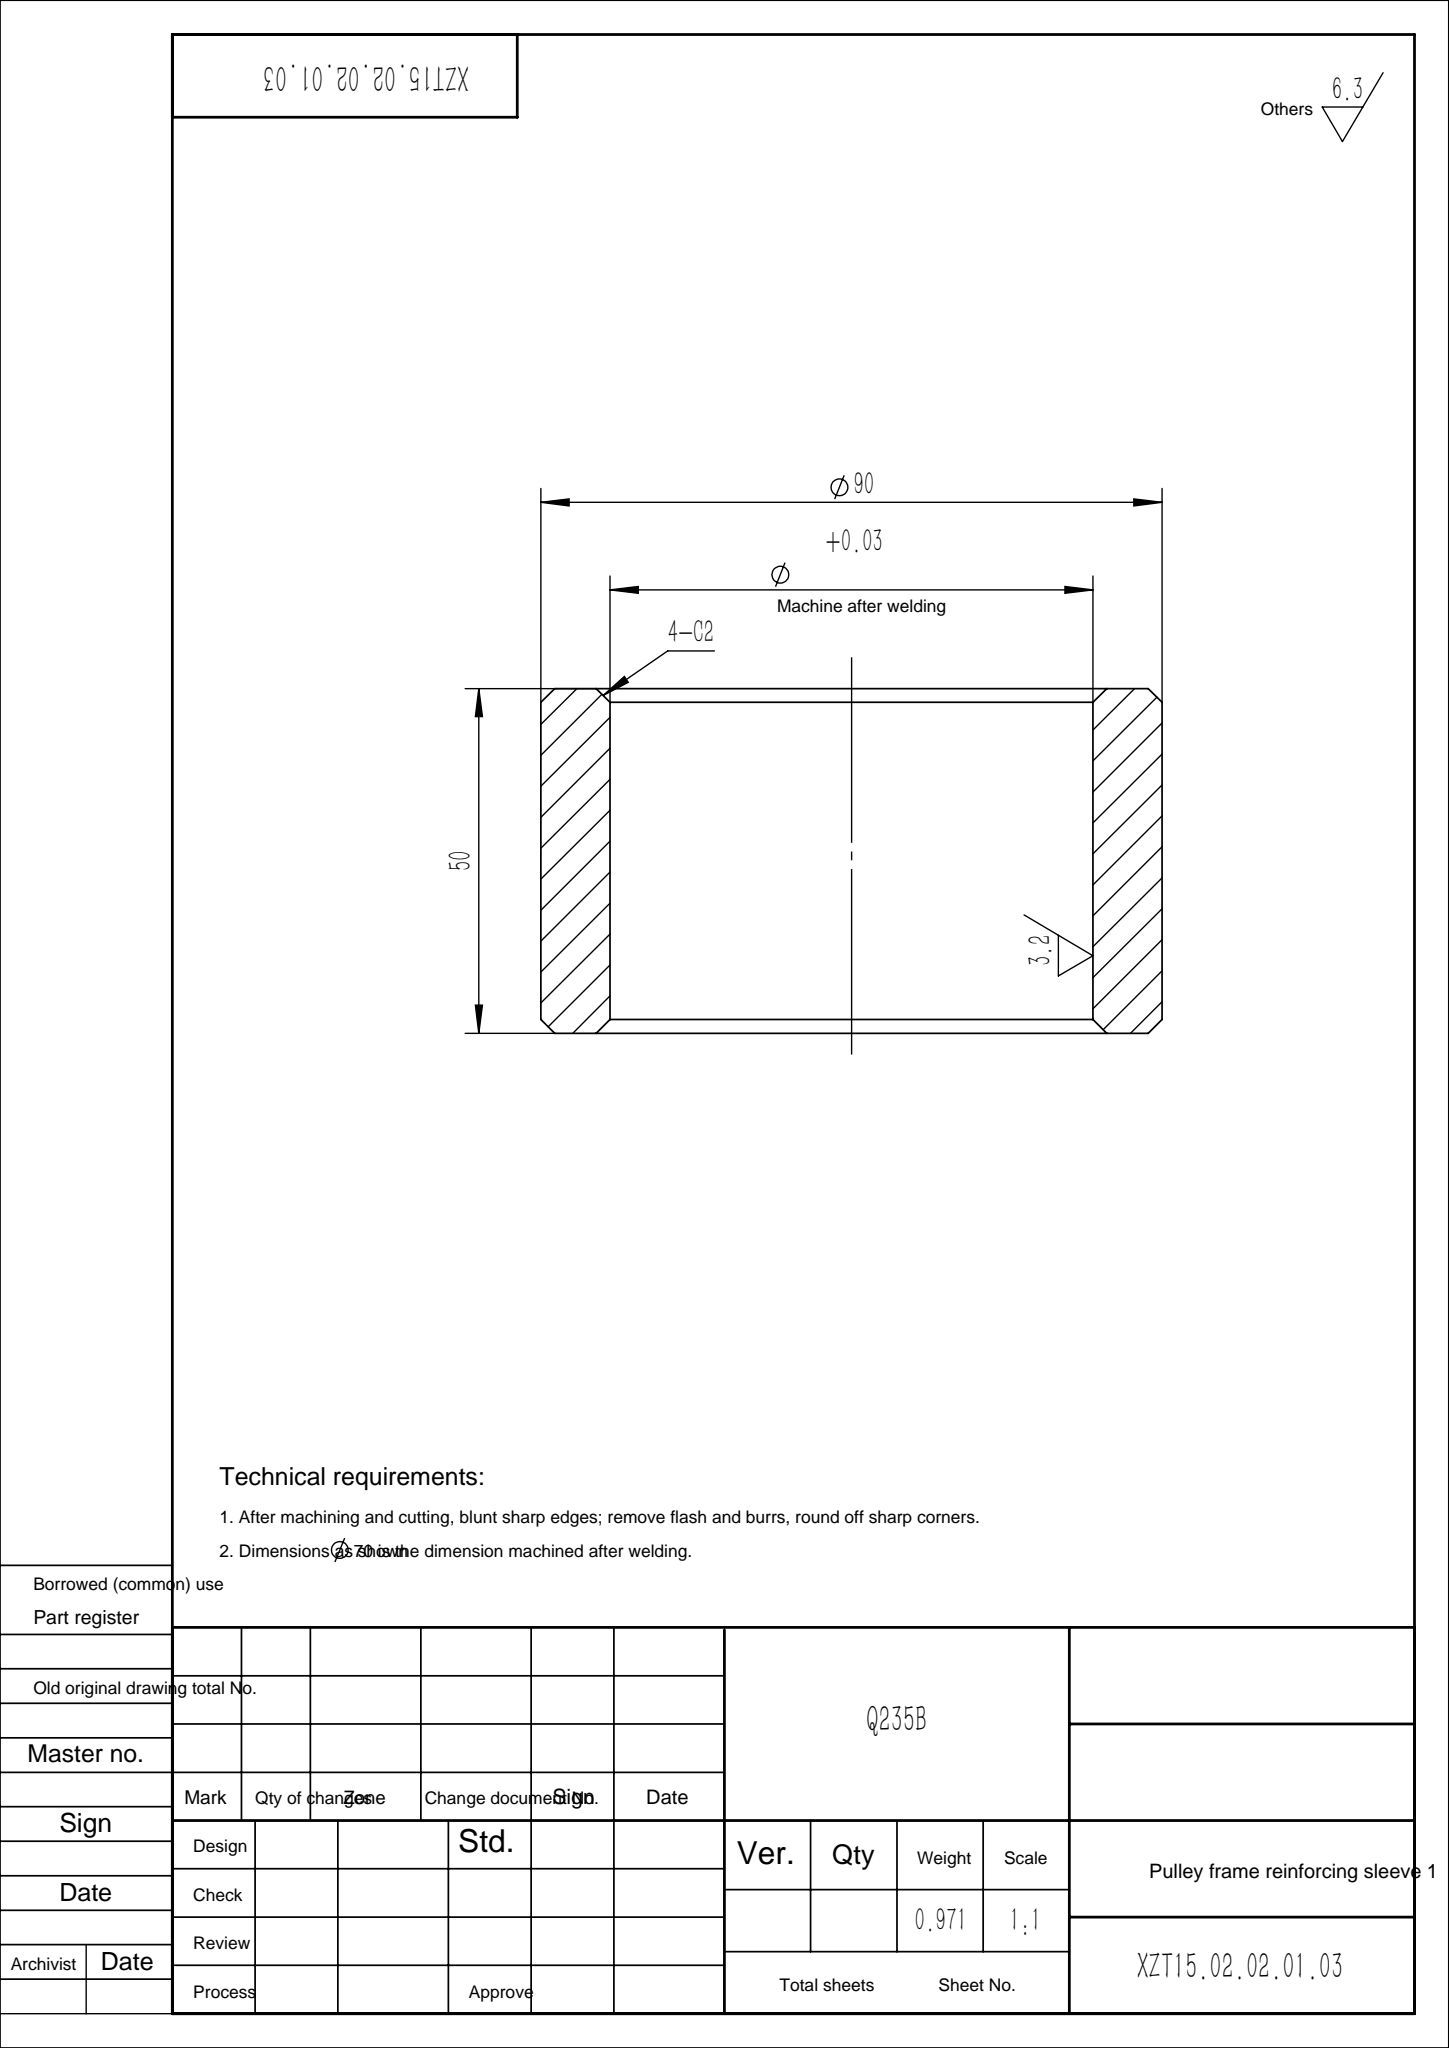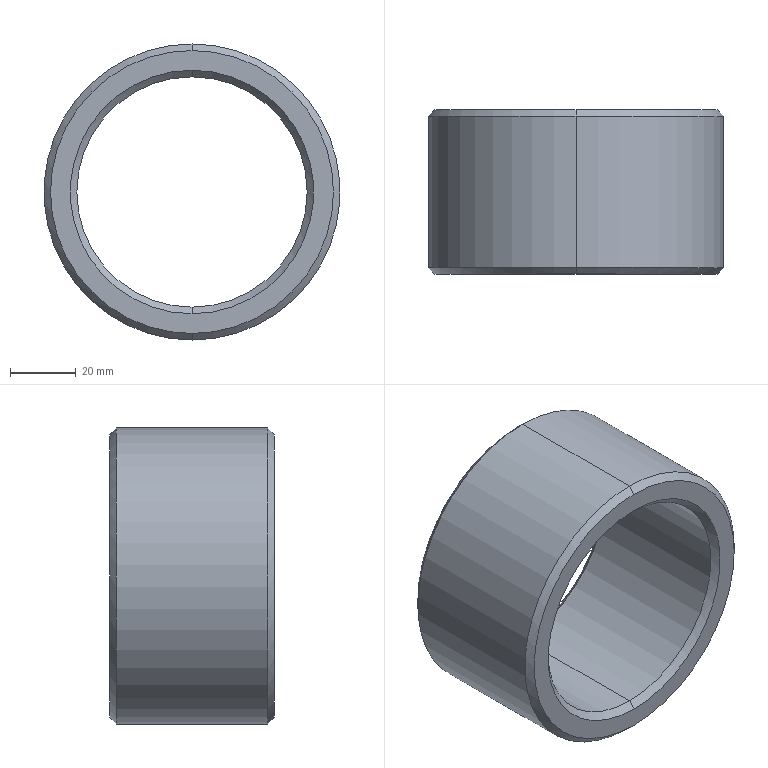Part | SolidWorks | features Chamfer 1, Extrusion 1 | 1 solid | 14 faces | box 90 x 50 x 90 mm | volume 123653 mm3 | cone 8 | cylinder 4 | plane 2 | commonest cylinder face diameters 70 x2 90 x2
STEP:
#1=CARTESIAN_POINT('',(0.,50.,43.));
#2=VERTEX_POINT('',#1);
#3=CARTESIAN_POINT('',(0.,50.,-43.));
#4=VERTEX_POINT('',#3);
#5=CARTESIAN_POINT('',(0.,50.,0.));
#6=DIRECTION('',(0.,1.,0.));
#7=DIRECTION('',(0.,0.,1.));
#8=AXIS2_PLACEMENT_3D('',#5,#6,#7);
#9=CIRCLE('',#8,43.);
#10=EDGE_CURVE('',#2,#4,#9,.T.);
#11=ORIENTED_EDGE('',*,*,#10,.F.);
#12=CARTESIAN_POINT('',(0.,48.,45.));
#13=VERTEX_POINT('',#12);
#14=CARTESIAN_POINT('',(0.,50.,43.));
#15=DIRECTION('',(0.,-0.7071,0.7071));
#16=VECTOR('',#15,1000.);
#17=LINE('',#14,#16);
#18=EDGE_CURVE('',#2,#13,#17,.T.);
#19=ORIENTED_EDGE('',*,*,#18,.T.);
#20=CARTESIAN_POINT('',(0.,48.,-45.));
#21=VERTEX_POINT('',#20);
#22=CARTESIAN_POINT('',(0.,48.,0.));
#23=DIRECTION('',(0.,-1.,0.));
#24=DIRECTION('',(0.,0.,1.));
#25=AXIS2_PLACEMENT_3D('',#22,#23,#24);
#26=CIRCLE('',#25,45.);
#27=EDGE_CURVE('',#21,#13,#26,.T.);
#28=ORIENTED_EDGE('',*,*,#27,.F.);
#29=CARTESIAN_POINT('',(0.,50.,-43.));
#30=DIRECTION('',(0.,-0.7071,-0.7071));
#31=VECTOR('',#30,1000.);
#32=LINE('',#29,#31);
#33=EDGE_CURVE('',#4,#21,#32,.T.);
#34=ORIENTED_EDGE('',*,*,#33,.F.);
#35=EDGE_LOOP('',(#11,#19,#28,#34));
#36=FACE_OUTER_BOUND('',#35,.T.);
#37=CARTESIAN_POINT('',(0.,50.,0.));
#38=DIRECTION('',(0.,-1.,0.));
#39=DIRECTION('',(0.,0.,-1.));
#40=AXIS2_PLACEMENT_3D('',#37,#38,#39);
#41=CONICAL_SURFACE('',#40,43.,0.7854);
#42=ADVANCED_FACE('',(#36),#41,.T.);
#43=CARTESIAN_POINT('',(0.,0.,-43.));
#44=VERTEX_POINT('',#43);
#45=CARTESIAN_POINT('',(0.,0.,43.));
#46=VERTEX_POINT('',#45);
#47=CARTESIAN_POINT('',(0.,0.,0.));
#48=DIRECTION('',(0.,-1.,0.));
#49=DIRECTION('',(0.,0.,1.));
#50=AXIS2_PLACEMENT_3D('',#47,#48,#49);
#51=CIRCLE('',#50,43.);
#52=EDGE_CURVE('',#44,#46,#51,.T.);
#53=ORIENTED_EDGE('',*,*,#52,.F.);
#54=CARTESIAN_POINT('',(0.,2.,-45.));
#55=VERTEX_POINT('',#54);
#56=CARTESIAN_POINT('',(0.,2.,-45.));
#57=DIRECTION('',(0.,0.7071,-0.7071));
#58=VECTOR('',#57,1000.);
#59=LINE('',#56,#58);
#60=EDGE_CURVE('',#44,#55,#59,.T.);
#61=ORIENTED_EDGE('',*,*,#60,.T.);
#62=CARTESIAN_POINT('',(0.,2.,45.));
#63=VERTEX_POINT('',#62);
#64=CARTESIAN_POINT('',(0.,2.,0.));
#65=DIRECTION('',(0.,1.,0.));
#66=DIRECTION('',(0.,0.,1.));
#67=AXIS2_PLACEMENT_3D('',#64,#65,#66);
#68=CIRCLE('',#67,45.);
#69=EDGE_CURVE('',#63,#55,#68,.T.);
#70=ORIENTED_EDGE('',*,*,#69,.F.);
#71=CARTESIAN_POINT('',(0.,2.,45.));
#72=DIRECTION('',(0.,0.7071,0.7071));
#73=VECTOR('',#72,1000.);
#74=LINE('',#71,#73);
#75=EDGE_CURVE('',#46,#63,#74,.T.);
#76=ORIENTED_EDGE('',*,*,#75,.F.);
#77=EDGE_LOOP('',(#53,#61,#70,#76));
#78=FACE_OUTER_BOUND('',#77,.T.);
#79=CARTESIAN_POINT('',(0.,2.,0.));
#80=DIRECTION('',(0.,1.,0.));
#81=DIRECTION('',(0.,0.,1.));
#82=AXIS2_PLACEMENT_3D('',#79,#80,#81);
#83=CONICAL_SURFACE('',#82,45.,0.7854);
#84=ADVANCED_FACE('',(#78),#83,.T.);
#85=CARTESIAN_POINT('',(0.,48.,-35.));
#86=VERTEX_POINT('',#85);
#87=CARTESIAN_POINT('',(0.,48.,35.));
#88=VERTEX_POINT('',#87);
#89=CARTESIAN_POINT('',(0.,48.,0.));
#90=DIRECTION('',(0.,1.,0.));
#91=DIRECTION('',(0.,0.,1.));
#92=AXIS2_PLACEMENT_3D('',#89,#90,#91);
#93=CIRCLE('',#92,35.);
#94=EDGE_CURVE('',#86,#88,#93,.T.);
#95=ORIENTED_EDGE('',*,*,#94,.F.);
#96=CARTESIAN_POINT('',(0.,50.,-37.));
#97=VERTEX_POINT('',#96);
#98=CARTESIAN_POINT('',(0.,48.,-35.));
#99=DIRECTION('',(0.,0.7071,-0.7071));
#100=VECTOR('',#99,1000.);
#101=LINE('',#98,#100);
#102=EDGE_CURVE('',#86,#97,#101,.T.);
#103=ORIENTED_EDGE('',*,*,#102,.T.);
#104=CARTESIAN_POINT('',(0.,50.,37.));
#105=VERTEX_POINT('',#104);
#106=CARTESIAN_POINT('',(0.,50.,0.));
#107=DIRECTION('',(0.,-1.,0.));
#108=DIRECTION('',(0.,0.,1.));
#109=AXIS2_PLACEMENT_3D('',#106,#107,#108);
#110=CIRCLE('',#109,37.);
#111=EDGE_CURVE('',#105,#97,#110,.T.);
#112=ORIENTED_EDGE('',*,*,#111,.F.);
#113=CARTESIAN_POINT('',(0.,48.,35.));
#114=DIRECTION('',(0.,0.7071,0.7071));
#115=VECTOR('',#114,1000.);
#116=LINE('',#113,#115);
#117=EDGE_CURVE('',#88,#105,#116,.T.);
#118=ORIENTED_EDGE('',*,*,#117,.F.);
#119=EDGE_LOOP('',(#95,#103,#112,#118));
#120=FACE_OUTER_BOUND('',#119,.T.);
#121=CARTESIAN_POINT('',(0.,48.,0.));
#122=DIRECTION('',(0.,1.,0.));
#123=DIRECTION('',(0.,0.,1.));
#124=AXIS2_PLACEMENT_3D('',#121,#122,#123);
#125=CONICAL_SURFACE('',#124,35.,0.7854);
#126=ADVANCED_FACE('',(#120),#125,.F.);
#127=CARTESIAN_POINT('',(0.,2.,35.));
#128=VERTEX_POINT('',#127);
#129=CARTESIAN_POINT('',(0.,2.,-35.));
#130=VERTEX_POINT('',#129);
#131=CARTESIAN_POINT('',(0.,2.,0.));
#132=DIRECTION('',(0.,-1.,0.));
#133=DIRECTION('',(0.,0.,1.));
#134=AXIS2_PLACEMENT_3D('',#131,#132,#133);
#135=CIRCLE('',#134,35.);
#136=EDGE_CURVE('',#128,#130,#135,.T.);
#137=ORIENTED_EDGE('',*,*,#136,.F.);
#138=CARTESIAN_POINT('',(0.,0.,37.));
#139=VERTEX_POINT('',#138);
#140=CARTESIAN_POINT('',(0.,0.,37.));
#141=DIRECTION('',(0.,-0.7071,0.7071));
#142=VECTOR('',#141,1000.);
#143=LINE('',#140,#142);
#144=EDGE_CURVE('',#128,#139,#143,.T.);
#145=ORIENTED_EDGE('',*,*,#144,.T.);
#146=CARTESIAN_POINT('',(0.,0.,-37.));
#147=VERTEX_POINT('',#146);
#148=CARTESIAN_POINT('',(0.,0.,0.));
#149=DIRECTION('',(0.,1.,0.));
#150=DIRECTION('',(0.,0.,1.));
#151=AXIS2_PLACEMENT_3D('',#148,#149,#150);
#152=CIRCLE('',#151,37.);
#153=EDGE_CURVE('',#147,#139,#152,.T.);
#154=ORIENTED_EDGE('',*,*,#153,.F.);
#155=CARTESIAN_POINT('',(0.,0.,-37.));
#156=DIRECTION('',(0.,-0.7071,-0.7071));
#157=VECTOR('',#156,1000.);
#158=LINE('',#155,#157);
#159=EDGE_CURVE('',#130,#147,#158,.T.);
#160=ORIENTED_EDGE('',*,*,#159,.F.);
#161=EDGE_LOOP('',(#137,#145,#154,#160));
#162=FACE_OUTER_BOUND('',#161,.T.);
#163=CARTESIAN_POINT('',(0.,0.,0.));
#164=DIRECTION('',(0.,-1.,0.));
#165=DIRECTION('',(0.,0.,-1.));
#166=AXIS2_PLACEMENT_3D('',#163,#164,#165);
#167=CONICAL_SURFACE('',#166,37.,0.7854);
#168=ADVANCED_FACE('',(#162),#167,.F.);
#169=ORIENTED_EDGE('',*,*,#94,.T.);
#170=CARTESIAN_POINT('',(0.,50.,35.));
#171=DIRECTION('',(0.,-1.,0.));
#172=VECTOR('',#171,1000.);
#173=LINE('',#170,#172);
#174=EDGE_CURVE('',#88,#128,#173,.T.);
#175=ORIENTED_EDGE('',*,*,#174,.T.);
#176=ORIENTED_EDGE('',*,*,#136,.T.);
#177=CARTESIAN_POINT('',(0.,50.,-35.));
#178=DIRECTION('',(0.,-1.,0.));
#179=VECTOR('',#178,1000.);
#180=LINE('',#177,#179);
#181=EDGE_CURVE('',#86,#130,#180,.T.);
#182=ORIENTED_EDGE('',*,*,#181,.F.);
#183=EDGE_LOOP('',(#169,#175,#176,#182));
#184=FACE_OUTER_BOUND('',#183,.T.);
#185=CARTESIAN_POINT('',(0.,50.,0.));
#186=DIRECTION('',(0.,-1.,0.));
#187=DIRECTION('',(0.,0.,-1.));
#188=AXIS2_PLACEMENT_3D('',#185,#186,#187);
#189=CYLINDRICAL_SURFACE('',#188,35.);
#190=ADVANCED_FACE('',(#184),#189,.F.);
#191=ORIENTED_EDGE('',*,*,#27,.T.);
#192=CARTESIAN_POINT('',(0.,50.,45.));
#193=DIRECTION('',(0.,-1.,0.));
#194=VECTOR('',#193,1000.);
#195=LINE('',#192,#194);
#196=EDGE_CURVE('',#13,#63,#195,.T.);
#197=ORIENTED_EDGE('',*,*,#196,.T.);
#198=ORIENTED_EDGE('',*,*,#69,.T.);
#199=CARTESIAN_POINT('',(0.,50.,-45.));
#200=DIRECTION('',(0.,-1.,0.));
#201=VECTOR('',#200,1000.);
#202=LINE('',#199,#201);
#203=EDGE_CURVE('',#21,#55,#202,.T.);
#204=ORIENTED_EDGE('',*,*,#203,.F.);
#205=EDGE_LOOP('',(#191,#197,#198,#204));
#206=FACE_OUTER_BOUND('',#205,.T.);
#207=CARTESIAN_POINT('',(0.,50.,0.));
#208=DIRECTION('',(0.,-1.,0.));
#209=DIRECTION('',(0.,0.,-1.));
#210=AXIS2_PLACEMENT_3D('',#207,#208,#209);
#211=CYLINDRICAL_SURFACE('',#210,45.);
#212=ADVANCED_FACE('',(#206),#211,.T.);
#213=ORIENTED_EDGE('',*,*,#111,.T.);
#214=CARTESIAN_POINT('',(0.,50.,0.));
#215=DIRECTION('',(0.,-1.,0.));
#216=DIRECTION('',(0.,0.,1.));
#217=AXIS2_PLACEMENT_3D('',#214,#215,#216);
#218=CIRCLE('',#217,37.);
#219=EDGE_CURVE('',#97,#105,#218,.T.);
#220=ORIENTED_EDGE('',*,*,#219,.T.);
#221=EDGE_LOOP('',(#213,#220));
#222=FACE_BOUND('',#221,.T.);
#223=CARTESIAN_POINT('',(0.,50.,0.));
#224=DIRECTION('',(0.,1.,0.));
#225=DIRECTION('',(0.,0.,1.));
#226=AXIS2_PLACEMENT_3D('',#223,#224,#225);
#227=CIRCLE('',#226,43.);
#228=EDGE_CURVE('',#4,#2,#227,.T.);
#229=ORIENTED_EDGE('',*,*,#228,.T.);
#230=ORIENTED_EDGE('',*,*,#10,.T.);
#231=EDGE_LOOP('',(#229,#230));
#232=FACE_OUTER_BOUND('',#231,.T.);
#233=CARTESIAN_POINT('',(0.,50.,0.));
#234=DIRECTION('',(0.,1.,0.));
#235=DIRECTION('',(0.,0.,1.));
#236=AXIS2_PLACEMENT_3D('',#233,#234,#235);
#237=PLANE('',#236);
#238=ADVANCED_FACE('',(#222,#232),#237,.T.);
#239=ORIENTED_EDGE('',*,*,#153,.T.);
#240=CARTESIAN_POINT('',(0.,0.,0.));
#241=DIRECTION('',(0.,1.,0.));
#242=DIRECTION('',(0.,0.,1.));
#243=AXIS2_PLACEMENT_3D('',#240,#241,#242);
#244=CIRCLE('',#243,37.);
#245=EDGE_CURVE('',#139,#147,#244,.T.);
#246=ORIENTED_EDGE('',*,*,#245,.T.);
#247=EDGE_LOOP('',(#239,#246));
#248=FACE_BOUND('',#247,.T.);
#249=CARTESIAN_POINT('',(0.,0.,0.));
#250=DIRECTION('',(0.,-1.,0.));
#251=DIRECTION('',(0.,0.,1.));
#252=AXIS2_PLACEMENT_3D('',#249,#250,#251);
#253=CIRCLE('',#252,43.);
#254=EDGE_CURVE('',#46,#44,#253,.T.);
#255=ORIENTED_EDGE('',*,*,#254,.T.);
#256=ORIENTED_EDGE('',*,*,#52,.T.);
#257=EDGE_LOOP('',(#255,#256));
#258=FACE_OUTER_BOUND('',#257,.T.);
#259=CARTESIAN_POINT('',(0.,0.,0.));
#260=DIRECTION('',(0.,1.,0.));
#261=DIRECTION('',(0.,0.,1.));
#262=AXIS2_PLACEMENT_3D('',#259,#260,#261);
#263=PLANE('',#262);
#264=ADVANCED_FACE('',(#248,#258),#263,.F.);
#265=ORIENTED_EDGE('',*,*,#196,.F.);
#266=CARTESIAN_POINT('',(0.,48.,0.));
#267=DIRECTION('',(0.,-1.,0.));
#268=DIRECTION('',(0.,0.,1.));
#269=AXIS2_PLACEMENT_3D('',#266,#267,#268);
#270=CIRCLE('',#269,45.);
#271=EDGE_CURVE('',#13,#21,#270,.T.);
#272=ORIENTED_EDGE('',*,*,#271,.T.);
#273=ORIENTED_EDGE('',*,*,#203,.T.);
#274=CARTESIAN_POINT('',(0.,2.,0.));
#275=DIRECTION('',(0.,1.,0.));
#276=DIRECTION('',(0.,0.,1.));
#277=AXIS2_PLACEMENT_3D('',#274,#275,#276);
#278=CIRCLE('',#277,45.);
#279=EDGE_CURVE('',#55,#63,#278,.T.);
#280=ORIENTED_EDGE('',*,*,#279,.T.);
#281=EDGE_LOOP('',(#265,#272,#273,#280));
#282=FACE_OUTER_BOUND('',#281,.T.);
#283=CARTESIAN_POINT('',(0.,50.,0.));
#284=DIRECTION('',(0.,-1.,0.));
#285=DIRECTION('',(0.,0.,-1.));
#286=AXIS2_PLACEMENT_3D('',#283,#284,#285);
#287=CYLINDRICAL_SURFACE('',#286,45.);
#288=ADVANCED_FACE('',(#282),#287,.T.);
#289=ORIENTED_EDGE('',*,*,#174,.F.);
#290=CARTESIAN_POINT('',(0.,48.,0.));
#291=DIRECTION('',(0.,1.,0.));
#292=DIRECTION('',(0.,0.,1.));
#293=AXIS2_PLACEMENT_3D('',#290,#291,#292);
#294=CIRCLE('',#293,35.);
#295=EDGE_CURVE('',#88,#86,#294,.T.);
#296=ORIENTED_EDGE('',*,*,#295,.T.);
#297=ORIENTED_EDGE('',*,*,#181,.T.);
#298=CARTESIAN_POINT('',(0.,2.,0.));
#299=DIRECTION('',(0.,-1.,0.));
#300=DIRECTION('',(0.,0.,1.));
#301=AXIS2_PLACEMENT_3D('',#298,#299,#300);
#302=CIRCLE('',#301,35.);
#303=EDGE_CURVE('',#130,#128,#302,.T.);
#304=ORIENTED_EDGE('',*,*,#303,.T.);
#305=EDGE_LOOP('',(#289,#296,#297,#304));
#306=FACE_OUTER_BOUND('',#305,.T.);
#307=CARTESIAN_POINT('',(0.,50.,0.));
#308=DIRECTION('',(0.,-1.,0.));
#309=DIRECTION('',(0.,0.,-1.));
#310=AXIS2_PLACEMENT_3D('',#307,#308,#309);
#311=CYLINDRICAL_SURFACE('',#310,35.);
#312=ADVANCED_FACE('',(#306),#311,.F.);
#313=ORIENTED_EDGE('',*,*,#144,.F.);
#314=ORIENTED_EDGE('',*,*,#303,.F.);
#315=ORIENTED_EDGE('',*,*,#159,.T.);
#316=ORIENTED_EDGE('',*,*,#245,.F.);
#317=EDGE_LOOP('',(#313,#314,#315,#316));
#318=FACE_OUTER_BOUND('',#317,.T.);
#319=CARTESIAN_POINT('',(0.,0.,0.));
#320=DIRECTION('',(0.,-1.,0.));
#321=DIRECTION('',(0.,0.,-1.));
#322=AXIS2_PLACEMENT_3D('',#319,#320,#321);
#323=CONICAL_SURFACE('',#322,37.,0.7854);
#324=ADVANCED_FACE('',(#318),#323,.F.);
#325=ORIENTED_EDGE('',*,*,#102,.F.);
#326=ORIENTED_EDGE('',*,*,#295,.F.);
#327=ORIENTED_EDGE('',*,*,#117,.T.);
#328=ORIENTED_EDGE('',*,*,#219,.F.);
#329=EDGE_LOOP('',(#325,#326,#327,#328));
#330=FACE_OUTER_BOUND('',#329,.T.);
#331=CARTESIAN_POINT('',(0.,48.,0.));
#332=DIRECTION('',(0.,1.,0.));
#333=DIRECTION('',(0.,0.,1.));
#334=AXIS2_PLACEMENT_3D('',#331,#332,#333);
#335=CONICAL_SURFACE('',#334,35.,0.7854);
#336=ADVANCED_FACE('',(#330),#335,.F.);
#337=ORIENTED_EDGE('',*,*,#60,.F.);
#338=ORIENTED_EDGE('',*,*,#254,.F.);
#339=ORIENTED_EDGE('',*,*,#75,.T.);
#340=ORIENTED_EDGE('',*,*,#279,.F.);
#341=EDGE_LOOP('',(#337,#338,#339,#340));
#342=FACE_OUTER_BOUND('',#341,.T.);
#343=CARTESIAN_POINT('',(0.,2.,0.));
#344=DIRECTION('',(0.,1.,0.));
#345=DIRECTION('',(0.,0.,1.));
#346=AXIS2_PLACEMENT_3D('',#343,#344,#345);
#347=CONICAL_SURFACE('',#346,45.,0.7854);
#348=ADVANCED_FACE('',(#342),#347,.T.);
#349=ORIENTED_EDGE('',*,*,#18,.F.);
#350=ORIENTED_EDGE('',*,*,#228,.F.);
#351=ORIENTED_EDGE('',*,*,#33,.T.);
#352=ORIENTED_EDGE('',*,*,#271,.F.);
#353=EDGE_LOOP('',(#349,#350,#351,#352));
#354=FACE_OUTER_BOUND('',#353,.T.);
#355=CARTESIAN_POINT('',(0.,50.,0.));
#356=DIRECTION('',(0.,-1.,0.));
#357=DIRECTION('',(0.,0.,-1.));
#358=AXIS2_PLACEMENT_3D('',#355,#356,#357);
#359=CONICAL_SURFACE('',#358,43.,0.7854);
#360=ADVANCED_FACE('',(#354),#359,.T.);
#361=CLOSED_SHELL('',(#42,#84,#126,#168,#190,#212,#238,#264,#288,#312,#324,#336,#348,#360));
#362=MANIFOLD_SOLID_BREP('',#361);
#363=CARTESIAN_POINT('',(0.,0.,0.));
#364=DIRECTION('',(0.,0.,1.));
#365=DIRECTION('',(1.,0.,0.));
#366=AXIS2_PLACEMENT_3D('',#363,#364,#365);
#367=(LENGTH_UNIT()NAMED_UNIT(*)SI_UNIT(.MILLI.,.METRE.));
#368=UNCERTAINTY_MEASURE_WITH_UNIT(LENGTH_MEASURE(0.00001),#367,'','');
#369=(NAMED_UNIT(*)PLANE_ANGLE_UNIT()SI_UNIT($,.RADIAN.));
#370=(NAMED_UNIT(*)SI_UNIT($,.STERADIAN.)SOLID_ANGLE_UNIT());
#371=(GEOMETRIC_REPRESENTATION_CONTEXT(3)GLOBAL_UNCERTAINTY_ASSIGNED_CONTEXT((#368))GLOBAL_UNIT_ASSIGNED_CONTEXT((#367,#369,#370))REPRESENTATION_CONTEXT('',''));
#372=ADVANCED_BREP_SHAPE_REPRESENTATION('',(#362,#366),#371);